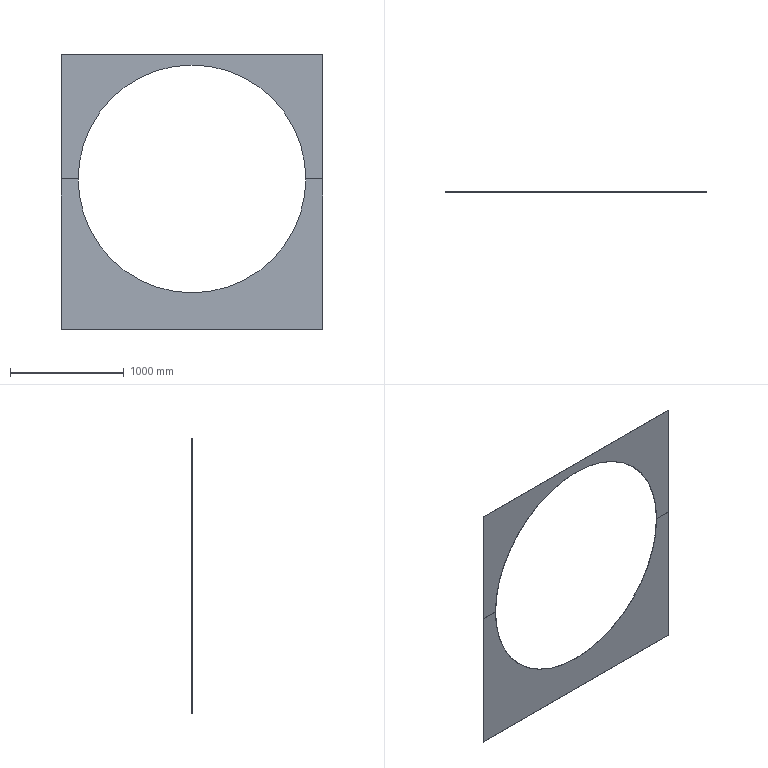Part | STEP file | Bracket checkered plate 8 | 2 solids | 17 faces | box 2300 x 3 x 2420 mm | volume 7273222 mm3 | plane 14 | cylinder 3 | commonest cylinder face diameters 2000 x3
STEP:
#1=CARTESIAN_POINT('',(0.,0.,0.));
#2=DIRECTION('',(0.,0.,1.));
#3=DIRECTION('',(1.,0.,0.));
#4=AXIS2_PLACEMENT_3D('',#1,#2,#3);
#5=CARTESIAN_POINT('',(2150.,3.,-1095.));
#6=VERTEX_POINT('',#5);
#7=CARTESIAN_POINT('',(2150.,0.,-1095.));
#8=VERTEX_POINT('',#7);
#9=CARTESIAN_POINT('',(2150.,-7.,-1095.));
#10=DIRECTION('',(0.,-1.,0.));
#11=VECTOR('',#10,1.);
#12=LINE('',#9,#11);
#13=CARTESIAN_POINT('',(1150.,-7.,-1095.));
#14=DIRECTION('',(0.,1.,0.));
#15=DIRECTION('',(0.,0.,1.));
#16=AXIS2_PLACEMENT_3D('',#13,#14,#15);
#17=CYLINDRICAL_SURFACE('',#16,1000.);
#18=CARTESIAN_POINT('',(1.571,0.));
#19=DIRECTION('',(0.,-1.));
#20=VECTOR('',#19,1.);
#21=LINE('',#18,#20);
#22=(GEOMETRIC_REPRESENTATION_CONTEXT(2)PARAMETRIC_REPRESENTATION_CONTEXT()REPRESENTATION_CONTEXT('',''));
#23=DEFINITIONAL_REPRESENTATION('',(#21),#22);
#24=PCURVE('',#17,#23);
#25=CARTESIAN_POINT('',(0.,-0.01,-1095.));
#26=DIRECTION('',(0.,0.,1.));
#27=DIRECTION('',(1.,0.,0.));
#28=AXIS2_PLACEMENT_3D('',#25,#26,#27);
#29=PLANE('',#28);
#30=CARTESIAN_POINT('',(2150.,-6.99));
#31=DIRECTION('',(0.,-1.));
#32=VECTOR('',#31,1.);
#33=LINE('',#30,#32);
#34=(GEOMETRIC_REPRESENTATION_CONTEXT(2)PARAMETRIC_REPRESENTATION_CONTEXT()REPRESENTATION_CONTEXT('',''));
#35=DEFINITIONAL_REPRESENTATION('',(#33),#34);
#36=PCURVE('',#29,#35);
#37=SURFACE_CURVE('',#12,(#24,#36),.PCURVE_S1.);
#38=EDGE_CURVE('',#6,#8,#37,.T.);
#39=ORIENTED_EDGE('',*,*,#38,.F.);
#40=CARTESIAN_POINT('',(1150.,3.,-95.));
#41=VERTEX_POINT('',#40);
#42=CARTESIAN_POINT('',(1150.,3.,-1095.));
#43=DIRECTION('',(0.,1.,0.));
#44=DIRECTION('',(0.,0.,1.));
#45=AXIS2_PLACEMENT_3D('',#42,#43,#44);
#46=CIRCLE('',#45,1000.);
#47=CARTESIAN_POINT('',(0.,10.));
#48=DIRECTION('',(1.,0.));
#49=VECTOR('',#48,1.);
#50=LINE('',#47,#49);
#51=(GEOMETRIC_REPRESENTATION_CONTEXT(2)PARAMETRIC_REPRESENTATION_CONTEXT()REPRESENTATION_CONTEXT('',''));
#52=DEFINITIONAL_REPRESENTATION('',(#50),#51);
#53=PCURVE('',#17,#52);
#54=CARTESIAN_POINT('',(0.,3.,0.));
#55=DIRECTION('',(0.,-1.,0.));
#56=DIRECTION('',(0.,0.,-1.));
#57=AXIS2_PLACEMENT_3D('',#54,#55,#56);
#58=PLANE('',#57);
#59=CARTESIAN_POINT('',(95.,1150.));
#60=CARTESIAN_POINT('',(95.,2882.051));
#61=CARTESIAN_POINT('',(1595.,2016.025));
#62=CARTESIAN_POINT('',(3095.,1150.));
#63=CARTESIAN_POINT('',(1595.,283.975));
#64=CARTESIAN_POINT('',(95.,-582.051));
#65=CARTESIAN_POINT('',(95.,1150.));
#66=(BOUNDED_CURVE()B_SPLINE_CURVE(2,(#59,#60,#61,#62,#63,#64,#65),.UNSPECIFIED.,.T.,.F.)B_SPLINE_CURVE_WITH_KNOTS((1,2,2,2,2,1),(-2.094,0.,2.094,4.189,6.283,8.378),.UNSPECIFIED.)CURVE()GEOMETRIC_REPRESENTATION_ITEM()RATIONAL_B_SPLINE_CURVE((1.,0.5,1.,0.5,1.,0.5,1.))REPRESENTATION_ITEM(''));
#67=(GEOMETRIC_REPRESENTATION_CONTEXT(2)PARAMETRIC_REPRESENTATION_CONTEXT()REPRESENTATION_CONTEXT('',''));
#68=DEFINITIONAL_REPRESENTATION('',(#66),#67);
#69=PCURVE('',#58,#68);
#70=SURFACE_CURVE('',#46,(#53,#69),.PCURVE_S1.);
#71=EDGE_CURVE('',#41,#6,#70,.T.);
#72=ORIENTED_EDGE('',*,*,#71,.F.);
#73=CARTESIAN_POINT('',(1150.,0.,-95.));
#74=VERTEX_POINT('',#73);
#75=CARTESIAN_POINT('',(1150.,-7.,-95.));
#76=DIRECTION('',(0.,1.,0.));
#77=VECTOR('',#76,1.);
#78=LINE('',#75,#77);
#79=CARTESIAN_POINT('',(0.,0.));
#80=DIRECTION('',(0.,1.));
#81=VECTOR('',#80,1.);
#82=LINE('',#79,#81);
#83=(GEOMETRIC_REPRESENTATION_CONTEXT(2)PARAMETRIC_REPRESENTATION_CONTEXT()REPRESENTATION_CONTEXT('',''));
#84=DEFINITIONAL_REPRESENTATION('',(#82),#83);
#85=PCURVE('',#17,#84);
#86=CARTESIAN_POINT('',(1150.,-7.,-1095.));
#87=DIRECTION('',(0.,1.,0.));
#88=DIRECTION('',(0.,0.,1.));
#89=AXIS2_PLACEMENT_3D('',#86,#87,#88);
#90=CYLINDRICAL_SURFACE('',#89,1000.);
#91=CARTESIAN_POINT('',(6.283,0.));
#92=DIRECTION('',(0.,1.));
#93=VECTOR('',#92,1.);
#94=LINE('',#91,#93);
#95=(GEOMETRIC_REPRESENTATION_CONTEXT(2)PARAMETRIC_REPRESENTATION_CONTEXT()REPRESENTATION_CONTEXT('',''));
#96=DEFINITIONAL_REPRESENTATION('',(#94),#95);
#97=PCURVE('',#90,#96);
#98=SURFACE_CURVE('',#78,(#85,#97),.PCURVE_S1.);
#99=EDGE_CURVE('',#74,#41,#98,.T.);
#100=ORIENTED_EDGE('',*,*,#99,.F.);
#101=CARTESIAN_POINT('',(1150.,0.,-1095.));
#102=DIRECTION('',(0.,-1.,0.));
#103=DIRECTION('',(0.,0.,-1.));
#104=AXIS2_PLACEMENT_3D('',#101,#102,#103);
#105=CIRCLE('',#104,1000.);
#106=CARTESIAN_POINT('',(3.142,7.));
#107=DIRECTION('',(-1.,0.));
#108=VECTOR('',#107,1.);
#109=LINE('',#106,#108);
#110=(GEOMETRIC_REPRESENTATION_CONTEXT(2)PARAMETRIC_REPRESENTATION_CONTEXT()REPRESENTATION_CONTEXT('',''));
#111=DEFINITIONAL_REPRESENTATION('',(#109),#110);
#112=PCURVE('',#17,#111);
#113=CARTESIAN_POINT('',(0.,0.,0.));
#114=DIRECTION('',(0.,-1.,0.));
#115=DIRECTION('',(0.,0.,-1.));
#116=AXIS2_PLACEMENT_3D('',#113,#114,#115);
#117=PLANE('',#116);
#118=CARTESIAN_POINT('',(1095.,1150.));
#119=DIRECTION('',(1.,0.));
#120=AXIS2_PLACEMENT_2D('',#118,#119);
#121=CIRCLE('',#120,1000.);
#122=(GEOMETRIC_REPRESENTATION_CONTEXT(2)PARAMETRIC_REPRESENTATION_CONTEXT()REPRESENTATION_CONTEXT('',''));
#123=DEFINITIONAL_REPRESENTATION('',(#121),#122);
#124=PCURVE('',#117,#123);
#125=SURFACE_CURVE('',#105,(#112,#124),.PCURVE_S1.);
#126=EDGE_CURVE('',#8,#74,#125,.T.);
#127=ORIENTED_EDGE('',*,*,#126,.F.);
#128=EDGE_LOOP('',(#39,#72,#100,#127));
#129=FACE_BOUND('',#128,.F.);
#130=ADVANCED_FACE('',(#129),#17,.F.);
#131=CARTESIAN_POINT('',(2300.,0.,-1095.));
#132=VERTEX_POINT('',#131);
#133=CARTESIAN_POINT('',(0.,0.,-1095.));
#134=DIRECTION('',(-1.,0.,0.));
#135=VECTOR('',#134,1.);
#136=LINE('',#133,#135);
#137=CARTESIAN_POINT('',(0.,0.01));
#138=DIRECTION('',(-1.,0.));
#139=VECTOR('',#138,1.);
#140=LINE('',#137,#139);
#141=(GEOMETRIC_REPRESENTATION_CONTEXT(2)PARAMETRIC_REPRESENTATION_CONTEXT()REPRESENTATION_CONTEXT('',''));
#142=DEFINITIONAL_REPRESENTATION('',(#140),#141);
#143=PCURVE('',#29,#142);
#144=CARTESIAN_POINT('',(1095.,0.));
#145=DIRECTION('',(0.,-1.));
#146=VECTOR('',#145,1.);
#147=LINE('',#144,#146);
#148=(GEOMETRIC_REPRESENTATION_CONTEXT(2)PARAMETRIC_REPRESENTATION_CONTEXT()REPRESENTATION_CONTEXT('',''));
#149=DEFINITIONAL_REPRESENTATION('',(#147),#148);
#150=PCURVE('',#117,#149);
#151=SURFACE_CURVE('',#136,(#143,#150),.PCURVE_S1.);
#152=EDGE_CURVE('',#132,#8,#151,.T.);
#153=ORIENTED_EDGE('',*,*,#152,.T.);
#154=ORIENTED_EDGE('',*,*,#38,.F.);
#155=CARTESIAN_POINT('',(2300.,3.,-1095.));
#156=VERTEX_POINT('',#155);
#157=CARTESIAN_POINT('',(0.,3.,-1095.));
#158=DIRECTION('',(-1.,0.,0.));
#159=VECTOR('',#158,1.);
#160=LINE('',#157,#159);
#161=CARTESIAN_POINT('',(0.,3.01));
#162=DIRECTION('',(-1.,0.));
#163=VECTOR('',#162,1.);
#164=LINE('',#161,#163);
#165=(GEOMETRIC_REPRESENTATION_CONTEXT(2)PARAMETRIC_REPRESENTATION_CONTEXT()REPRESENTATION_CONTEXT('',''));
#166=DEFINITIONAL_REPRESENTATION('',(#164),#165);
#167=PCURVE('',#29,#166);
#168=CARTESIAN_POINT('',(1095.,0.));
#169=DIRECTION('',(0.,-1.));
#170=VECTOR('',#169,1.);
#171=LINE('',#168,#170);
#172=(GEOMETRIC_REPRESENTATION_CONTEXT(2)PARAMETRIC_REPRESENTATION_CONTEXT()REPRESENTATION_CONTEXT('',''));
#173=DEFINITIONAL_REPRESENTATION('',(#171),#172);
#174=PCURVE('',#58,#173);
#175=SURFACE_CURVE('',#160,(#167,#174),.PCURVE_S1.);
#176=EDGE_CURVE('',#156,#6,#175,.T.);
#177=ORIENTED_EDGE('',*,*,#176,.F.);
#178=CARTESIAN_POINT('',(2300.,3.,-1095.));
#179=DIRECTION('',(0.,1.,0.));
#180=VECTOR('',#179,1.);
#181=LINE('',#178,#180);
#182=CARTESIAN_POINT('',(2300.,3.01));
#183=DIRECTION('',(0.,1.));
#184=VECTOR('',#183,1.);
#185=LINE('',#182,#184);
#186=(GEOMETRIC_REPRESENTATION_CONTEXT(2)PARAMETRIC_REPRESENTATION_CONTEXT()REPRESENTATION_CONTEXT('',''));
#187=DEFINITIONAL_REPRESENTATION('',(#185),#186);
#188=PCURVE('',#29,#187);
#189=CARTESIAN_POINT('',(2300.,3.,0.));
#190=DIRECTION('',(-1.,0.,0.));
#191=DIRECTION('',(0.,0.,1.));
#192=AXIS2_PLACEMENT_3D('',#189,#190,#191);
#193=PLANE('',#192);
#194=CARTESIAN_POINT('',(-1095.,0.));
#195=DIRECTION('',(0.,1.));
#196=VECTOR('',#195,1.);
#197=LINE('',#194,#196);
#198=(GEOMETRIC_REPRESENTATION_CONTEXT(2)PARAMETRIC_REPRESENTATION_CONTEXT()REPRESENTATION_CONTEXT('',''));
#199=DEFINITIONAL_REPRESENTATION('',(#197),#198);
#200=PCURVE('',#193,#199);
#201=SURFACE_CURVE('',#181,(#188,#200),.PCURVE_S1.);
#202=EDGE_CURVE('',#132,#156,#201,.T.);
#203=ORIENTED_EDGE('',*,*,#202,.F.);
#204=EDGE_LOOP('',(#153,#154,#177,#203));
#205=FACE_BOUND('',#204,.T.);
#206=ADVANCED_FACE('',(#205),#29,.F.);
#207=CARTESIAN_POINT('',(150.,0.,-1095.));
#208=VERTEX_POINT('',#207);
#209=CARTESIAN_POINT('',(0.,0.,-1095.));
#210=VERTEX_POINT('',#209);
#211=CARTESIAN_POINT('',(0.,0.,-1095.));
#212=DIRECTION('',(-1.,0.,0.));
#213=VECTOR('',#212,1.);
#214=LINE('',#211,#213);
#215=CARTESIAN_POINT('',(0.,-0.01,-1095.));
#216=DIRECTION('',(0.,0.,1.));
#217=DIRECTION('',(1.,0.,0.));
#218=AXIS2_PLACEMENT_3D('',#215,#216,#217);
#219=PLANE('',#218);
#220=CARTESIAN_POINT('',(0.,0.01));
#221=DIRECTION('',(-1.,0.));
#222=VECTOR('',#221,1.);
#223=LINE('',#220,#222);
#224=(GEOMETRIC_REPRESENTATION_CONTEXT(2)PARAMETRIC_REPRESENTATION_CONTEXT()REPRESENTATION_CONTEXT('',''));
#225=DEFINITIONAL_REPRESENTATION('',(#223),#224);
#226=PCURVE('',#219,#225);
#227=CARTESIAN_POINT('',(1095.,0.));
#228=DIRECTION('',(0.,-1.));
#229=VECTOR('',#228,1.);
#230=LINE('',#227,#229);
#231=(GEOMETRIC_REPRESENTATION_CONTEXT(2)PARAMETRIC_REPRESENTATION_CONTEXT()REPRESENTATION_CONTEXT('',''));
#232=DEFINITIONAL_REPRESENTATION('',(#230),#231);
#233=PCURVE('',#117,#232);
#234=SURFACE_CURVE('',#214,(#226,#233),.PCURVE_S1.);
#235=EDGE_CURVE('',#208,#210,#234,.T.);
#236=ORIENTED_EDGE('',*,*,#235,.T.);
#237=CARTESIAN_POINT('',(0.,3.,-1095.));
#238=VERTEX_POINT('',#237);
#239=CARTESIAN_POINT('',(0.,3.,-1095.));
#240=DIRECTION('',(0.,-1.,0.));
#241=VECTOR('',#240,1.);
#242=LINE('',#239,#241);
#243=CARTESIAN_POINT('',(0.,3.01));
#244=DIRECTION('',(0.,-1.));
#245=VECTOR('',#244,1.);
#246=LINE('',#243,#245);
#247=(GEOMETRIC_REPRESENTATION_CONTEXT(2)PARAMETRIC_REPRESENTATION_CONTEXT()REPRESENTATION_CONTEXT('',''));
#248=DEFINITIONAL_REPRESENTATION('',(#246),#247);
#249=PCURVE('',#219,#248);
#250=CARTESIAN_POINT('',(0.,3.,0.));
#251=DIRECTION('',(1.,0.,0.));
#252=DIRECTION('',(0.,0.,-1.));
#253=AXIS2_PLACEMENT_3D('',#250,#251,#252);
#254=PLANE('',#253);
#255=CARTESIAN_POINT('',(1095.,0.));
#256=DIRECTION('',(0.,-1.));
#257=VECTOR('',#256,1.);
#258=LINE('',#255,#257);
#259=(GEOMETRIC_REPRESENTATION_CONTEXT(2)PARAMETRIC_REPRESENTATION_CONTEXT()REPRESENTATION_CONTEXT('',''));
#260=DEFINITIONAL_REPRESENTATION('',(#258),#259);
#261=PCURVE('',#254,#260);
#262=SURFACE_CURVE('',#242,(#249,#261),.PCURVE_S1.);
#263=EDGE_CURVE('',#238,#210,#262,.T.);
#264=ORIENTED_EDGE('',*,*,#263,.F.);
#265=CARTESIAN_POINT('',(150.,3.,-1095.));
#266=VERTEX_POINT('',#265);
#267=CARTESIAN_POINT('',(0.,3.,-1095.));
#268=DIRECTION('',(-1.,0.,0.));
#269=VECTOR('',#268,1.);
#270=LINE('',#267,#269);
#271=CARTESIAN_POINT('',(0.,3.01));
#272=DIRECTION('',(-1.,0.));
#273=VECTOR('',#272,1.);
#274=LINE('',#271,#273);
#275=(GEOMETRIC_REPRESENTATION_CONTEXT(2)PARAMETRIC_REPRESENTATION_CONTEXT()REPRESENTATION_CONTEXT('',''));
#276=DEFINITIONAL_REPRESENTATION('',(#274),#275);
#277=PCURVE('',#219,#276);
#278=CARTESIAN_POINT('',(1095.,0.));
#279=DIRECTION('',(0.,-1.));
#280=VECTOR('',#279,1.);
#281=LINE('',#278,#280);
#282=(GEOMETRIC_REPRESENTATION_CONTEXT(2)PARAMETRIC_REPRESENTATION_CONTEXT()REPRESENTATION_CONTEXT('',''));
#283=DEFINITIONAL_REPRESENTATION('',(#281),#282);
#284=PCURVE('',#58,#283);
#285=SURFACE_CURVE('',#270,(#277,#284),.PCURVE_S1.);
#286=EDGE_CURVE('',#266,#238,#285,.T.);
#287=ORIENTED_EDGE('',*,*,#286,.F.);
#288=CARTESIAN_POINT('',(150.,-7.,-1095.));
#289=DIRECTION('',(0.,1.,0.));
#290=VECTOR('',#289,1.);
#291=LINE('',#288,#290);
#292=CARTESIAN_POINT('',(150.,-6.99));
#293=DIRECTION('',(0.,1.));
#294=VECTOR('',#293,1.);
#295=LINE('',#292,#294);
#296=(GEOMETRIC_REPRESENTATION_CONTEXT(2)PARAMETRIC_REPRESENTATION_CONTEXT()REPRESENTATION_CONTEXT('',''));
#297=DEFINITIONAL_REPRESENTATION('',(#295),#296);
#298=PCURVE('',#219,#297);
#299=CARTESIAN_POINT('',(4.712,0.));
#300=DIRECTION('',(0.,1.));
#301=VECTOR('',#300,1.);
#302=LINE('',#299,#301);
#303=(GEOMETRIC_REPRESENTATION_CONTEXT(2)PARAMETRIC_REPRESENTATION_CONTEXT()REPRESENTATION_CONTEXT('',''));
#304=DEFINITIONAL_REPRESENTATION('',(#302),#303);
#305=PCURVE('',#90,#304);
#306=SURFACE_CURVE('',#291,(#298,#305),.PCURVE_S1.);
#307=EDGE_CURVE('',#208,#266,#306,.T.);
#308=ORIENTED_EDGE('',*,*,#307,.F.);
#309=EDGE_LOOP('',(#236,#264,#287,#308));
#310=FACE_BOUND('',#309,.T.);
#311=ADVANCED_FACE('',(#310),#219,.F.);
#312=CARTESIAN_POINT('',(1150.,3.,-1095.));
#313=DIRECTION('',(0.,1.,0.));
#314=DIRECTION('',(0.,0.,1.));
#315=AXIS2_PLACEMENT_3D('',#312,#313,#314);
#316=CIRCLE('',#315,1000.);
#317=CARTESIAN_POINT('',(0.,10.));
#318=DIRECTION('',(1.,0.));
#319=VECTOR('',#318,1.);
#320=LINE('',#317,#319);
#321=(GEOMETRIC_REPRESENTATION_CONTEXT(2)PARAMETRIC_REPRESENTATION_CONTEXT()REPRESENTATION_CONTEXT('',''));
#322=DEFINITIONAL_REPRESENTATION('',(#320),#321);
#323=PCURVE('',#90,#322);
#324=CARTESIAN_POINT('',(95.,1150.));
#325=CARTESIAN_POINT('',(95.,2882.051));
#326=CARTESIAN_POINT('',(1595.,2016.025));
#327=CARTESIAN_POINT('',(3095.,1150.));
#328=CARTESIAN_POINT('',(1595.,283.975));
#329=CARTESIAN_POINT('',(95.,-582.051));
#330=CARTESIAN_POINT('',(95.,1150.));
#331=(BOUNDED_CURVE()B_SPLINE_CURVE(2,(#324,#325,#326,#327,#328,#329,#330),.UNSPECIFIED.,.T.,.F.)B_SPLINE_CURVE_WITH_KNOTS((1,2,2,2,2,1),(-2.094,0.,2.094,4.189,6.283,8.378),.UNSPECIFIED.)CURVE()GEOMETRIC_REPRESENTATION_ITEM()RATIONAL_B_SPLINE_CURVE((1.,0.5,1.,0.5,1.,0.5,1.))REPRESENTATION_ITEM(''));
#332=(GEOMETRIC_REPRESENTATION_CONTEXT(2)PARAMETRIC_REPRESENTATION_CONTEXT()REPRESENTATION_CONTEXT('',''));
#333=DEFINITIONAL_REPRESENTATION('',(#331),#332);
#334=PCURVE('',#58,#333);
#335=SURFACE_CURVE('',#316,(#323,#334),.PCURVE_S1.);
#336=EDGE_CURVE('',#266,#41,#335,.T.);
#337=ORIENTED_EDGE('',*,*,#336,.F.);
#338=ORIENTED_EDGE('',*,*,#307,.F.);
#339=CARTESIAN_POINT('',(1150.,0.,-1095.));
#340=DIRECTION('',(0.,-1.,0.));
#341=DIRECTION('',(0.,0.,-1.));
#342=AXIS2_PLACEMENT_3D('',#339,#340,#341);
#343=CIRCLE('',#342,1000.);
#344=CARTESIAN_POINT('',(9.425,7.));
#345=DIRECTION('',(-1.,0.));
#346=VECTOR('',#345,1.);
#347=LINE('',#344,#346);
#348=(GEOMETRIC_REPRESENTATION_CONTEXT(2)PARAMETRIC_REPRESENTATION_CONTEXT()REPRESENTATION_CONTEXT('',''));
#349=DEFINITIONAL_REPRESENTATION('',(#347),#348);
#350=PCURVE('',#90,#349);
#351=CARTESIAN_POINT('',(1095.,1150.));
#352=DIRECTION('',(1.,0.));
#353=AXIS2_PLACEMENT_2D('',#351,#352);
#354=CIRCLE('',#353,1000.);
#355=(GEOMETRIC_REPRESENTATION_CONTEXT(2)PARAMETRIC_REPRESENTATION_CONTEXT()REPRESENTATION_CONTEXT('',''));
#356=DEFINITIONAL_REPRESENTATION('',(#354),#355);
#357=PCURVE('',#117,#356);
#358=SURFACE_CURVE('',#343,(#350,#357),.PCURVE_S1.);
#359=EDGE_CURVE('',#74,#208,#358,.T.);
#360=ORIENTED_EDGE('',*,*,#359,.F.);
#361=ORIENTED_EDGE('',*,*,#99,.T.);
#362=EDGE_LOOP('',(#337,#338,#360,#361));
#363=FACE_BOUND('',#362,.F.);
#364=ADVANCED_FACE('',(#363),#90,.F.);
#365=CARTESIAN_POINT('',(2300.,3.,0.));
#366=VERTEX_POINT('',#365);
#367=CARTESIAN_POINT('',(2300.,3.,0.));
#368=DIRECTION('',(0.,0.,-1.));
#369=VECTOR('',#368,1.);
#370=LINE('',#367,#369);
#371=CARTESIAN_POINT('',(0.,2300.));
#372=DIRECTION('',(1.,0.));
#373=VECTOR('',#372,1.);
#374=LINE('',#371,#373);
#375=(GEOMETRIC_REPRESENTATION_CONTEXT(2)PARAMETRIC_REPRESENTATION_CONTEXT()REPRESENTATION_CONTEXT('',''));
#376=DEFINITIONAL_REPRESENTATION('',(#374),#375);
#377=PCURVE('',#58,#376);
#378=CARTESIAN_POINT('',(0.,0.));
#379=DIRECTION('',(-1.,0.));
#380=VECTOR('',#379,1.);
#381=LINE('',#378,#380);
#382=(GEOMETRIC_REPRESENTATION_CONTEXT(2)PARAMETRIC_REPRESENTATION_CONTEXT()REPRESENTATION_CONTEXT('',''));
#383=DEFINITIONAL_REPRESENTATION('',(#381),#382);
#384=PCURVE('',#193,#383);
#385=SURFACE_CURVE('',#370,(#377,#384),.PCURVE_S1.);
#386=EDGE_CURVE('',#366,#156,#385,.T.);
#387=ORIENTED_EDGE('',*,*,#386,.T.);
#388=ORIENTED_EDGE('',*,*,#176,.T.);
#389=ORIENTED_EDGE('',*,*,#71,.F.);
#390=ORIENTED_EDGE('',*,*,#336,.F.);
#391=ORIENTED_EDGE('',*,*,#286,.T.);
#392=CARTESIAN_POINT('',(0.,3.,0.));
#393=VERTEX_POINT('',#392);
#394=CARTESIAN_POINT('',(0.,3.,0.));
#395=DIRECTION('',(0.,0.,1.));
#396=VECTOR('',#395,1.);
#397=LINE('',#394,#396);
#398=CARTESIAN_POINT('',(0.,0.));
#399=DIRECTION('',(-1.,0.));
#400=VECTOR('',#399,1.);
#401=LINE('',#398,#400);
#402=(GEOMETRIC_REPRESENTATION_CONTEXT(2)PARAMETRIC_REPRESENTATION_CONTEXT()REPRESENTATION_CONTEXT('',''));
#403=DEFINITIONAL_REPRESENTATION('',(#401),#402);
#404=PCURVE('',#58,#403);
#405=CARTESIAN_POINT('',(0.,0.));
#406=DIRECTION('',(-1.,0.));
#407=VECTOR('',#406,1.);
#408=LINE('',#405,#407);
#409=(GEOMETRIC_REPRESENTATION_CONTEXT(2)PARAMETRIC_REPRESENTATION_CONTEXT()REPRESENTATION_CONTEXT('',''));
#410=DEFINITIONAL_REPRESENTATION('',(#408),#409);
#411=PCURVE('',#254,#410);
#412=SURFACE_CURVE('',#397,(#404,#411),.PCURVE_S1.);
#413=EDGE_CURVE('',#238,#393,#412,.T.);
#414=ORIENTED_EDGE('',*,*,#413,.T.);
#415=CARTESIAN_POINT('',(0.,3.,0.));
#416=DIRECTION('',(1.,0.,0.));
#417=VECTOR('',#416,1.);
#418=LINE('',#415,#417);
#419=CARTESIAN_POINT('',(0.,0.));
#420=DIRECTION('',(0.,1.));
#421=VECTOR('',#420,1.);
#422=LINE('',#419,#421);
#423=(GEOMETRIC_REPRESENTATION_CONTEXT(2)PARAMETRIC_REPRESENTATION_CONTEXT()REPRESENTATION_CONTEXT('',''));
#424=DEFINITIONAL_REPRESENTATION('',(#422),#423);
#425=PCURVE('',#58,#424);
#426=CARTESIAN_POINT('',(0.,3.,0.));
#427=DIRECTION('',(0.,0.,-1.));
#428=DIRECTION('',(-1.,0.,0.));
#429=AXIS2_PLACEMENT_3D('',#426,#427,#428);
#430=PLANE('',#429);
#431=CARTESIAN_POINT('',(0.,0.));
#432=DIRECTION('',(-1.,0.));
#433=VECTOR('',#432,1.);
#434=LINE('',#431,#433);
#435=(GEOMETRIC_REPRESENTATION_CONTEXT(2)PARAMETRIC_REPRESENTATION_CONTEXT()REPRESENTATION_CONTEXT('',''));
#436=DEFINITIONAL_REPRESENTATION('',(#434),#435);
#437=PCURVE('',#430,#436);
#438=SURFACE_CURVE('',#418,(#425,#437),.PCURVE_S1.);
#439=EDGE_CURVE('',#393,#366,#438,.T.);
#440=ORIENTED_EDGE('',*,*,#439,.T.);
#441=EDGE_LOOP('',(#387,#388,#389,#390,#391,#414,#440));
#442=FACE_BOUND('',#441,.T.);
#443=ADVANCED_FACE('',(#442),#58,.F.);
#444=ORIENTED_EDGE('',*,*,#152,.F.);
#445=CARTESIAN_POINT('',(2300.,0.,0.));
#446=VERTEX_POINT('',#445);
#447=CARTESIAN_POINT('',(2300.,0.,0.));
#448=DIRECTION('',(0.,0.,-1.));
#449=VECTOR('',#448,1.);
#450=LINE('',#447,#449);
#451=CARTESIAN_POINT('',(0.,2300.));
#452=DIRECTION('',(1.,0.));
#453=VECTOR('',#452,1.);
#454=LINE('',#451,#453);
#455=(GEOMETRIC_REPRESENTATION_CONTEXT(2)PARAMETRIC_REPRESENTATION_CONTEXT()REPRESENTATION_CONTEXT('',''));
#456=DEFINITIONAL_REPRESENTATION('',(#454),#455);
#457=PCURVE('',#117,#456);
#458=CARTESIAN_POINT('',(0.,-3.));
#459=DIRECTION('',(-1.,0.));
#460=VECTOR('',#459,1.);
#461=LINE('',#458,#460);
#462=(GEOMETRIC_REPRESENTATION_CONTEXT(2)PARAMETRIC_REPRESENTATION_CONTEXT()REPRESENTATION_CONTEXT('',''));
#463=DEFINITIONAL_REPRESENTATION('',(#461),#462);
#464=PCURVE('',#193,#463);
#465=SURFACE_CURVE('',#450,(#457,#464),.PCURVE_S1.);
#466=EDGE_CURVE('',#446,#132,#465,.T.);
#467=ORIENTED_EDGE('',*,*,#466,.F.);
#468=CARTESIAN_POINT('',(0.,0.,0.));
#469=VERTEX_POINT('',#468);
#470=CARTESIAN_POINT('',(0.,0.,0.));
#471=DIRECTION('',(1.,0.,0.));
#472=VECTOR('',#471,1.);
#473=LINE('',#470,#472);
#474=CARTESIAN_POINT('',(0.,0.));
#475=DIRECTION('',(0.,1.));
#476=VECTOR('',#475,1.);
#477=LINE('',#474,#476);
#478=(GEOMETRIC_REPRESENTATION_CONTEXT(2)PARAMETRIC_REPRESENTATION_CONTEXT()REPRESENTATION_CONTEXT('',''));
#479=DEFINITIONAL_REPRESENTATION('',(#477),#478);
#480=PCURVE('',#117,#479);
#481=CARTESIAN_POINT('',(0.,-3.));
#482=DIRECTION('',(-1.,0.));
#483=VECTOR('',#482,1.);
#484=LINE('',#481,#483);
#485=(GEOMETRIC_REPRESENTATION_CONTEXT(2)PARAMETRIC_REPRESENTATION_CONTEXT()REPRESENTATION_CONTEXT('',''));
#486=DEFINITIONAL_REPRESENTATION('',(#484),#485);
#487=PCURVE('',#430,#486);
#488=SURFACE_CURVE('',#473,(#480,#487),.PCURVE_S1.);
#489=EDGE_CURVE('',#469,#446,#488,.T.);
#490=ORIENTED_EDGE('',*,*,#489,.F.);
#491=CARTESIAN_POINT('',(0.,0.,0.));
#492=DIRECTION('',(0.,0.,1.));
#493=VECTOR('',#492,1.);
#494=LINE('',#491,#493);
#495=CARTESIAN_POINT('',(0.,0.));
#496=DIRECTION('',(-1.,0.));
#497=VECTOR('',#496,1.);
#498=LINE('',#495,#497);
#499=(GEOMETRIC_REPRESENTATION_CONTEXT(2)PARAMETRIC_REPRESENTATION_CONTEXT()REPRESENTATION_CONTEXT('',''));
#500=DEFINITIONAL_REPRESENTATION('',(#498),#499);
#501=PCURVE('',#117,#500);
#502=CARTESIAN_POINT('',(0.,-3.));
#503=DIRECTION('',(-1.,0.));
#504=VECTOR('',#503,1.);
#505=LINE('',#502,#504);
#506=(GEOMETRIC_REPRESENTATION_CONTEXT(2)PARAMETRIC_REPRESENTATION_CONTEXT()REPRESENTATION_CONTEXT('',''));
#507=DEFINITIONAL_REPRESENTATION('',(#505),#506);
#508=PCURVE('',#254,#507);
#509=SURFACE_CURVE('',#494,(#501,#508),.PCURVE_S1.);
#510=EDGE_CURVE('',#210,#469,#509,.T.);
#511=ORIENTED_EDGE('',*,*,#510,.F.);
#512=ORIENTED_EDGE('',*,*,#235,.F.);
#513=ORIENTED_EDGE('',*,*,#359,.F.);
#514=ORIENTED_EDGE('',*,*,#126,.F.);
#515=EDGE_LOOP('',(#444,#467,#490,#511,#512,#513,#514));
#516=FACE_BOUND('',#515,.T.);
#517=ADVANCED_FACE('',(#516),#117,.T.);
#518=ORIENTED_EDGE('',*,*,#466,.T.);
#519=ORIENTED_EDGE('',*,*,#202,.T.);
#520=ORIENTED_EDGE('',*,*,#386,.F.);
#521=CARTESIAN_POINT('',(2300.,3.,0.));
#522=DIRECTION('',(0.,-1.,0.));
#523=VECTOR('',#522,1.);
#524=LINE('',#521,#523);
#525=CARTESIAN_POINT('',(0.,0.));
#526=DIRECTION('',(0.,-1.));
#527=VECTOR('',#526,1.);
#528=LINE('',#525,#527);
#529=(GEOMETRIC_REPRESENTATION_CONTEXT(2)PARAMETRIC_REPRESENTATION_CONTEXT()REPRESENTATION_CONTEXT('',''));
#530=DEFINITIONAL_REPRESENTATION('',(#528),#529);
#531=PCURVE('',#193,#530);
#532=CARTESIAN_POINT('',(-2300.,0.));
#533=DIRECTION('',(0.,-1.));
#534=VECTOR('',#533,1.);
#535=LINE('',#532,#534);
#536=(GEOMETRIC_REPRESENTATION_CONTEXT(2)PARAMETRIC_REPRESENTATION_CONTEXT()REPRESENTATION_CONTEXT('',''));
#537=DEFINITIONAL_REPRESENTATION('',(#535),#536);
#538=PCURVE('',#430,#537);
#539=SURFACE_CURVE('',#524,(#531,#538),.PCURVE_S1.);
#540=EDGE_CURVE('',#366,#446,#539,.T.);
#541=ORIENTED_EDGE('',*,*,#540,.T.);
#542=EDGE_LOOP('',(#518,#519,#520,#541));
#543=FACE_BOUND('',#542,.T.);
#544=ADVANCED_FACE('',(#543),#193,.F.);
#545=ORIENTED_EDGE('',*,*,#489,.T.);
#546=ORIENTED_EDGE('',*,*,#540,.F.);
#547=ORIENTED_EDGE('',*,*,#439,.F.);
#548=CARTESIAN_POINT('',(0.,3.,0.));
#549=DIRECTION('',(0.,-1.,0.));
#550=VECTOR('',#549,1.);
#551=LINE('',#548,#550);
#552=CARTESIAN_POINT('',(0.,0.));
#553=DIRECTION('',(0.,-1.));
#554=VECTOR('',#553,1.);
#555=LINE('',#552,#554);
#556=(GEOMETRIC_REPRESENTATION_CONTEXT(2)PARAMETRIC_REPRESENTATION_CONTEXT()REPRESENTATION_CONTEXT('',''));
#557=DEFINITIONAL_REPRESENTATION('',(#555),#556);
#558=PCURVE('',#430,#557);
#559=CARTESIAN_POINT('',(0.,0.));
#560=DIRECTION('',(0.,-1.));
#561=VECTOR('',#560,1.);
#562=LINE('',#559,#561);
#563=(GEOMETRIC_REPRESENTATION_CONTEXT(2)PARAMETRIC_REPRESENTATION_CONTEXT()REPRESENTATION_CONTEXT('',''));
#564=DEFINITIONAL_REPRESENTATION('',(#562),#563);
#565=PCURVE('',#254,#564);
#566=SURFACE_CURVE('',#551,(#558,#565),.PCURVE_S1.);
#567=EDGE_CURVE('',#393,#469,#566,.T.);
#568=ORIENTED_EDGE('',*,*,#567,.T.);
#569=EDGE_LOOP('',(#545,#546,#547,#568));
#570=FACE_BOUND('',#569,.T.);
#571=ADVANCED_FACE('',(#570),#430,.F.);
#572=ORIENTED_EDGE('',*,*,#413,.F.);
#573=ORIENTED_EDGE('',*,*,#263,.T.);
#574=ORIENTED_EDGE('',*,*,#510,.T.);
#575=ORIENTED_EDGE('',*,*,#567,.F.);
#576=EDGE_LOOP('',(#572,#573,#574,#575));
#577=FACE_BOUND('',#576,.T.);
#578=ADVANCED_FACE('',(#577),#254,.F.);
#579=CLOSED_SHELL('',(#130,#206,#311,#364,#443,#517,#544,#571,#578));
#580=MANIFOLD_SOLID_BREP('',#579);
#581=CARTESIAN_POINT('',(0.,3.,-1095.));
#582=VERTEX_POINT('',#581);
#583=CARTESIAN_POINT('',(0.,0.,-1095.));
#584=VERTEX_POINT('',#583);
#585=CARTESIAN_POINT('',(0.,3.,-1095.));
#586=DIRECTION('',(0.,-1.,0.));
#587=VECTOR('',#586,1.);
#588=LINE('',#585,#587);
#589=CARTESIAN_POINT('',(0.,3.,0.));
#590=DIRECTION('',(1.,0.,0.));
#591=DIRECTION('',(0.,0.,-1.));
#592=AXIS2_PLACEMENT_3D('',#589,#590,#591);
#593=PLANE('',#592);
#594=CARTESIAN_POINT('',(1095.,0.));
#595=DIRECTION('',(0.,-1.));
#596=VECTOR('',#595,1.);
#597=LINE('',#594,#596);
#598=(GEOMETRIC_REPRESENTATION_CONTEXT(2)PARAMETRIC_REPRESENTATION_CONTEXT()REPRESENTATION_CONTEXT('',''));
#599=DEFINITIONAL_REPRESENTATION('',(#597),#598);
#600=PCURVE('',#593,#599);
#601=CARTESIAN_POINT('',(0.,-0.01,-1095.));
#602=DIRECTION('',(0.,0.,1.));
#603=DIRECTION('',(1.,0.,0.));
#604=AXIS2_PLACEMENT_3D('',#601,#602,#603);
#605=PLANE('',#604);
#606=CARTESIAN_POINT('',(0.,3.01));
#607=DIRECTION('',(0.,-1.));
#608=VECTOR('',#607,1.);
#609=LINE('',#606,#608);
#610=(GEOMETRIC_REPRESENTATION_CONTEXT(2)PARAMETRIC_REPRESENTATION_CONTEXT()REPRESENTATION_CONTEXT('',''));
#611=DEFINITIONAL_REPRESENTATION('',(#609),#610);
#612=PCURVE('',#605,#611);
#613=SURFACE_CURVE('',#588,(#600,#612),.PCURVE_S1.);
#614=EDGE_CURVE('',#582,#584,#613,.T.);
#615=ORIENTED_EDGE('',*,*,#614,.F.);
#616=CARTESIAN_POINT('',(0.,3.,-2420.));
#617=VERTEX_POINT('',#616);
#618=CARTESIAN_POINT('',(0.,3.,0.));
#619=DIRECTION('',(0.,0.,1.));
#620=VECTOR('',#619,1.);
#621=LINE('',#618,#620);
#622=CARTESIAN_POINT('',(0.,0.));
#623=DIRECTION('',(-1.,0.));
#624=VECTOR('',#623,1.);
#625=LINE('',#622,#624);
#626=(GEOMETRIC_REPRESENTATION_CONTEXT(2)PARAMETRIC_REPRESENTATION_CONTEXT()REPRESENTATION_CONTEXT('',''));
#627=DEFINITIONAL_REPRESENTATION('',(#625),#626);
#628=PCURVE('',#593,#627);
#629=CARTESIAN_POINT('',(0.,3.,0.));
#630=DIRECTION('',(0.,-1.,0.));
#631=DIRECTION('',(0.,0.,-1.));
#632=AXIS2_PLACEMENT_3D('',#629,#630,#631);
#633=PLANE('',#632);
#634=CARTESIAN_POINT('',(0.,0.));
#635=DIRECTION('',(-1.,0.));
#636=VECTOR('',#635,1.);
#637=LINE('',#634,#636);
#638=(GEOMETRIC_REPRESENTATION_CONTEXT(2)PARAMETRIC_REPRESENTATION_CONTEXT()REPRESENTATION_CONTEXT('',''));
#639=DEFINITIONAL_REPRESENTATION('',(#637),#638);
#640=PCURVE('',#633,#639);
#641=SURFACE_CURVE('',#621,(#628,#640),.PCURVE_S1.);
#642=EDGE_CURVE('',#617,#582,#641,.T.);
#643=ORIENTED_EDGE('',*,*,#642,.F.);
#644=CARTESIAN_POINT('',(0.,0.,-2420.));
#645=VERTEX_POINT('',#644);
#646=CARTESIAN_POINT('',(0.,3.,-2420.));
#647=DIRECTION('',(0.,-1.,0.));
#648=VECTOR('',#647,1.);
#649=LINE('',#646,#648);
#650=CARTESIAN_POINT('',(2420.,0.));
#651=DIRECTION('',(0.,-1.));
#652=VECTOR('',#651,1.);
#653=LINE('',#650,#652);
#654=(GEOMETRIC_REPRESENTATION_CONTEXT(2)PARAMETRIC_REPRESENTATION_CONTEXT()REPRESENTATION_CONTEXT('',''));
#655=DEFINITIONAL_REPRESENTATION('',(#653),#654);
#656=PCURVE('',#593,#655);
#657=CARTESIAN_POINT('',(0.,3.,-2420.));
#658=DIRECTION('',(0.,0.,1.));
#659=DIRECTION('',(1.,0.,0.));
#660=AXIS2_PLACEMENT_3D('',#657,#658,#659);
#661=PLANE('',#660);
#662=CARTESIAN_POINT('',(0.,0.));
#663=DIRECTION('',(0.,-1.));
#664=VECTOR('',#663,1.);
#665=LINE('',#662,#664);
#666=(GEOMETRIC_REPRESENTATION_CONTEXT(2)PARAMETRIC_REPRESENTATION_CONTEXT()REPRESENTATION_CONTEXT('',''));
#667=DEFINITIONAL_REPRESENTATION('',(#665),#666);
#668=PCURVE('',#661,#667);
#669=SURFACE_CURVE('',#649,(#656,#668),.PCURVE_S1.);
#670=EDGE_CURVE('',#617,#645,#669,.T.);
#671=ORIENTED_EDGE('',*,*,#670,.T.);
#672=CARTESIAN_POINT('',(0.,0.,0.));
#673=DIRECTION('',(0.,0.,1.));
#674=VECTOR('',#673,1.);
#675=LINE('',#672,#674);
#676=CARTESIAN_POINT('',(0.,-3.));
#677=DIRECTION('',(-1.,0.));
#678=VECTOR('',#677,1.);
#679=LINE('',#676,#678);
#680=(GEOMETRIC_REPRESENTATION_CONTEXT(2)PARAMETRIC_REPRESENTATION_CONTEXT()REPRESENTATION_CONTEXT('',''));
#681=DEFINITIONAL_REPRESENTATION('',(#679),#680);
#682=PCURVE('',#593,#681);
#683=CARTESIAN_POINT('',(0.,0.,0.));
#684=DIRECTION('',(0.,-1.,0.));
#685=DIRECTION('',(0.,0.,-1.));
#686=AXIS2_PLACEMENT_3D('',#683,#684,#685);
#687=PLANE('',#686);
#688=CARTESIAN_POINT('',(0.,0.));
#689=DIRECTION('',(-1.,0.));
#690=VECTOR('',#689,1.);
#691=LINE('',#688,#690);
#692=(GEOMETRIC_REPRESENTATION_CONTEXT(2)PARAMETRIC_REPRESENTATION_CONTEXT()REPRESENTATION_CONTEXT('',''));
#693=DEFINITIONAL_REPRESENTATION('',(#691),#692);
#694=PCURVE('',#687,#693);
#695=SURFACE_CURVE('',#675,(#682,#694),.PCURVE_S1.);
#696=EDGE_CURVE('',#645,#584,#695,.T.);
#697=ORIENTED_EDGE('',*,*,#696,.T.);
#698=EDGE_LOOP('',(#615,#643,#671,#697));
#699=FACE_BOUND('',#698,.T.);
#700=ADVANCED_FACE('',(#699),#593,.F.);
#701=CARTESIAN_POINT('',(2300.,0.,-1095.));
#702=VERTEX_POINT('',#701);
#703=CARTESIAN_POINT('',(2300.,3.,-1095.));
#704=VERTEX_POINT('',#703);
#705=CARTESIAN_POINT('',(2300.,3.,-1095.));
#706=DIRECTION('',(0.,1.,0.));
#707=VECTOR('',#706,1.);
#708=LINE('',#705,#707);
#709=CARTESIAN_POINT('',(2300.,3.,0.));
#710=DIRECTION('',(-1.,0.,0.));
#711=DIRECTION('',(0.,0.,1.));
#712=AXIS2_PLACEMENT_3D('',#709,#710,#711);
#713=PLANE('',#712);
#714=CARTESIAN_POINT('',(-1095.,0.));
#715=DIRECTION('',(0.,1.));
#716=VECTOR('',#715,1.);
#717=LINE('',#714,#716);
#718=(GEOMETRIC_REPRESENTATION_CONTEXT(2)PARAMETRIC_REPRESENTATION_CONTEXT()REPRESENTATION_CONTEXT('',''));
#719=DEFINITIONAL_REPRESENTATION('',(#717),#718);
#720=PCURVE('',#713,#719);
#721=CARTESIAN_POINT('',(0.,-0.01,-1095.));
#722=DIRECTION('',(0.,0.,1.));
#723=DIRECTION('',(1.,0.,0.));
#724=AXIS2_PLACEMENT_3D('',#721,#722,#723);
#725=PLANE('',#724);
#726=CARTESIAN_POINT('',(2300.,3.01));
#727=DIRECTION('',(0.,1.));
#728=VECTOR('',#727,1.);
#729=LINE('',#726,#728);
#730=(GEOMETRIC_REPRESENTATION_CONTEXT(2)PARAMETRIC_REPRESENTATION_CONTEXT()REPRESENTATION_CONTEXT('',''));
#731=DEFINITIONAL_REPRESENTATION('',(#729),#730);
#732=PCURVE('',#725,#731);
#733=SURFACE_CURVE('',#708,(#720,#732),.PCURVE_S1.);
#734=EDGE_CURVE('',#702,#704,#733,.T.);
#735=ORIENTED_EDGE('',*,*,#734,.F.);
#736=CARTESIAN_POINT('',(2300.,0.,-2420.));
#737=VERTEX_POINT('',#736);
#738=CARTESIAN_POINT('',(2300.,0.,0.));
#739=DIRECTION('',(0.,0.,-1.));
#740=VECTOR('',#739,1.);
#741=LINE('',#738,#740);
#742=CARTESIAN_POINT('',(0.,-3.));
#743=DIRECTION('',(-1.,0.));
#744=VECTOR('',#743,1.);
#745=LINE('',#742,#744);
#746=(GEOMETRIC_REPRESENTATION_CONTEXT(2)PARAMETRIC_REPRESENTATION_CONTEXT()REPRESENTATION_CONTEXT('',''));
#747=DEFINITIONAL_REPRESENTATION('',(#745),#746);
#748=PCURVE('',#713,#747);
#749=CARTESIAN_POINT('',(0.,2300.));
#750=DIRECTION('',(1.,0.));
#751=VECTOR('',#750,1.);
#752=LINE('',#749,#751);
#753=(GEOMETRIC_REPRESENTATION_CONTEXT(2)PARAMETRIC_REPRESENTATION_CONTEXT()REPRESENTATION_CONTEXT('',''));
#754=DEFINITIONAL_REPRESENTATION('',(#752),#753);
#755=PCURVE('',#687,#754);
#756=SURFACE_CURVE('',#741,(#748,#755),.PCURVE_S1.);
#757=EDGE_CURVE('',#702,#737,#756,.T.);
#758=ORIENTED_EDGE('',*,*,#757,.T.);
#759=CARTESIAN_POINT('',(2300.,3.,-2420.));
#760=VERTEX_POINT('',#759);
#761=CARTESIAN_POINT('',(2300.,3.,-2420.));
#762=DIRECTION('',(0.,-1.,0.));
#763=VECTOR('',#762,1.);
#764=LINE('',#761,#763);
#765=CARTESIAN_POINT('',(-2420.,0.));
#766=DIRECTION('',(0.,-1.));
#767=VECTOR('',#766,1.);
#768=LINE('',#765,#767);
#769=(GEOMETRIC_REPRESENTATION_CONTEXT(2)PARAMETRIC_REPRESENTATION_CONTEXT()REPRESENTATION_CONTEXT('',''));
#770=DEFINITIONAL_REPRESENTATION('',(#768),#769);
#771=PCURVE('',#713,#770);
#772=CARTESIAN_POINT('',(2300.,0.));
#773=DIRECTION('',(0.,-1.));
#774=VECTOR('',#773,1.);
#775=LINE('',#772,#774);
#776=(GEOMETRIC_REPRESENTATION_CONTEXT(2)PARAMETRIC_REPRESENTATION_CONTEXT()REPRESENTATION_CONTEXT('',''));
#777=DEFINITIONAL_REPRESENTATION('',(#775),#776);
#778=PCURVE('',#661,#777);
#779=SURFACE_CURVE('',#764,(#771,#778),.PCURVE_S1.);
#780=EDGE_CURVE('',#760,#737,#779,.T.);
#781=ORIENTED_EDGE('',*,*,#780,.F.);
#782=CARTESIAN_POINT('',(2300.,3.,0.));
#783=DIRECTION('',(0.,0.,-1.));
#784=VECTOR('',#783,1.);
#785=LINE('',#782,#784);
#786=CARTESIAN_POINT('',(0.,0.));
#787=DIRECTION('',(-1.,0.));
#788=VECTOR('',#787,1.);
#789=LINE('',#786,#788);
#790=(GEOMETRIC_REPRESENTATION_CONTEXT(2)PARAMETRIC_REPRESENTATION_CONTEXT()REPRESENTATION_CONTEXT('',''));
#791=DEFINITIONAL_REPRESENTATION('',(#789),#790);
#792=PCURVE('',#713,#791);
#793=CARTESIAN_POINT('',(0.,2300.));
#794=DIRECTION('',(1.,0.));
#795=VECTOR('',#794,1.);
#796=LINE('',#793,#795);
#797=(GEOMETRIC_REPRESENTATION_CONTEXT(2)PARAMETRIC_REPRESENTATION_CONTEXT()REPRESENTATION_CONTEXT('',''));
#798=DEFINITIONAL_REPRESENTATION('',(#796),#797);
#799=PCURVE('',#633,#798);
#800=SURFACE_CURVE('',#785,(#792,#799),.PCURVE_S1.);
#801=EDGE_CURVE('',#704,#760,#800,.T.);
#802=ORIENTED_EDGE('',*,*,#801,.F.);
#803=EDGE_LOOP('',(#735,#758,#781,#802));
#804=FACE_BOUND('',#803,.T.);
#805=ADVANCED_FACE('',(#804),#713,.F.);
#806=CARTESIAN_POINT('',(2150.,3.,-1095.));
#807=VERTEX_POINT('',#806);
#808=CARTESIAN_POINT('',(0.,3.,-1095.));
#809=DIRECTION('',(-1.,0.,0.));
#810=VECTOR('',#809,1.);
#811=LINE('',#808,#810);
#812=CARTESIAN_POINT('',(1095.,0.));
#813=DIRECTION('',(0.,-1.));
#814=VECTOR('',#813,1.);
#815=LINE('',#812,#814);
#816=(GEOMETRIC_REPRESENTATION_CONTEXT(2)PARAMETRIC_REPRESENTATION_CONTEXT()REPRESENTATION_CONTEXT('',''));
#817=DEFINITIONAL_REPRESENTATION('',(#815),#816);
#818=PCURVE('',#633,#817);
#819=CARTESIAN_POINT('',(0.,3.01));
#820=DIRECTION('',(-1.,0.));
#821=VECTOR('',#820,1.);
#822=LINE('',#819,#821);
#823=(GEOMETRIC_REPRESENTATION_CONTEXT(2)PARAMETRIC_REPRESENTATION_CONTEXT()REPRESENTATION_CONTEXT('',''));
#824=DEFINITIONAL_REPRESENTATION('',(#822),#823);
#825=PCURVE('',#725,#824);
#826=SURFACE_CURVE('',#811,(#818,#825),.PCURVE_S1.);
#827=EDGE_CURVE('',#704,#807,#826,.T.);
#828=ORIENTED_EDGE('',*,*,#827,.F.);
#829=ORIENTED_EDGE('',*,*,#801,.T.);
#830=CARTESIAN_POINT('',(0.,3.,-2420.));
#831=DIRECTION('',(-1.,0.,0.));
#832=VECTOR('',#831,1.);
#833=LINE('',#830,#832);
#834=CARTESIAN_POINT('',(2420.,0.));
#835=DIRECTION('',(0.,-1.));
#836=VECTOR('',#835,1.);
#837=LINE('',#834,#836);
#838=(GEOMETRIC_REPRESENTATION_CONTEXT(2)PARAMETRIC_REPRESENTATION_CONTEXT()REPRESENTATION_CONTEXT('',''));
#839=DEFINITIONAL_REPRESENTATION('',(#837),#838);
#840=PCURVE('',#633,#839);
#841=CARTESIAN_POINT('',(0.,0.));
#842=DIRECTION('',(-1.,0.));
#843=VECTOR('',#842,1.);
#844=LINE('',#841,#843);
#845=(GEOMETRIC_REPRESENTATION_CONTEXT(2)PARAMETRIC_REPRESENTATION_CONTEXT()REPRESENTATION_CONTEXT('',''));
#846=DEFINITIONAL_REPRESENTATION('',(#844),#845);
#847=PCURVE('',#661,#846);
#848=SURFACE_CURVE('',#833,(#840,#847),.PCURVE_S1.);
#849=EDGE_CURVE('',#760,#617,#848,.T.);
#850=ORIENTED_EDGE('',*,*,#849,.T.);
#851=ORIENTED_EDGE('',*,*,#642,.T.);
#852=CARTESIAN_POINT('',(150.,3.,-1095.));
#853=VERTEX_POINT('',#852);
#854=CARTESIAN_POINT('',(0.,3.,-1095.));
#855=DIRECTION('',(-1.,0.,0.));
#856=VECTOR('',#855,1.);
#857=LINE('',#854,#856);
#858=CARTESIAN_POINT('',(1095.,0.));
#859=DIRECTION('',(0.,-1.));
#860=VECTOR('',#859,1.);
#861=LINE('',#858,#860);
#862=(GEOMETRIC_REPRESENTATION_CONTEXT(2)PARAMETRIC_REPRESENTATION_CONTEXT()REPRESENTATION_CONTEXT('',''));
#863=DEFINITIONAL_REPRESENTATION('',(#861),#862);
#864=PCURVE('',#633,#863);
#865=CARTESIAN_POINT('',(0.,3.01));
#866=DIRECTION('',(-1.,0.));
#867=VECTOR('',#866,1.);
#868=LINE('',#865,#867);
#869=(GEOMETRIC_REPRESENTATION_CONTEXT(2)PARAMETRIC_REPRESENTATION_CONTEXT()REPRESENTATION_CONTEXT('',''));
#870=DEFINITIONAL_REPRESENTATION('',(#868),#869);
#871=PCURVE('',#605,#870);
#872=SURFACE_CURVE('',#857,(#864,#871),.PCURVE_S1.);
#873=EDGE_CURVE('',#853,#582,#872,.T.);
#874=ORIENTED_EDGE('',*,*,#873,.F.);
#875=CARTESIAN_POINT('',(1150.,3.,-1095.));
#876=DIRECTION('',(0.,1.,0.));
#877=DIRECTION('',(0.,0.,1.));
#878=AXIS2_PLACEMENT_3D('',#875,#876,#877);
#879=CIRCLE('',#878,1000.);
#880=CARTESIAN_POINT('',(95.,1150.));
#881=CARTESIAN_POINT('',(95.,2882.051));
#882=CARTESIAN_POINT('',(1595.,2016.025));
#883=CARTESIAN_POINT('',(3095.,1150.));
#884=CARTESIAN_POINT('',(1595.,283.975));
#885=CARTESIAN_POINT('',(95.,-582.051));
#886=CARTESIAN_POINT('',(95.,1150.));
#887=(BOUNDED_CURVE()B_SPLINE_CURVE(2,(#880,#881,#882,#883,#884,#885,#886),.UNSPECIFIED.,.T.,.F.)B_SPLINE_CURVE_WITH_KNOTS((1,2,2,2,2,1),(-2.094,0.,2.094,4.189,6.283,8.378),.UNSPECIFIED.)CURVE()GEOMETRIC_REPRESENTATION_ITEM()RATIONAL_B_SPLINE_CURVE((1.,0.5,1.,0.5,1.,0.5,1.))REPRESENTATION_ITEM(''));
#888=(GEOMETRIC_REPRESENTATION_CONTEXT(2)PARAMETRIC_REPRESENTATION_CONTEXT()REPRESENTATION_CONTEXT('',''));
#889=DEFINITIONAL_REPRESENTATION('',(#887),#888);
#890=PCURVE('',#633,#889);
#891=CARTESIAN_POINT('',(1150.,-7.,-1095.));
#892=DIRECTION('',(0.,1.,0.));
#893=DIRECTION('',(0.,0.,1.));
#894=AXIS2_PLACEMENT_3D('',#891,#892,#893);
#895=CYLINDRICAL_SURFACE('',#894,1000.);
#896=CARTESIAN_POINT('',(0.,10.));
#897=DIRECTION('',(1.,0.));
#898=VECTOR('',#897,1.);
#899=LINE('',#896,#898);
#900=(GEOMETRIC_REPRESENTATION_CONTEXT(2)PARAMETRIC_REPRESENTATION_CONTEXT()REPRESENTATION_CONTEXT('',''));
#901=DEFINITIONAL_REPRESENTATION('',(#899),#900);
#902=PCURVE('',#895,#901);
#903=SURFACE_CURVE('',#879,(#890,#902),.PCURVE_S1.);
#904=EDGE_CURVE('',#807,#853,#903,.T.);
#905=ORIENTED_EDGE('',*,*,#904,.F.);
#906=EDGE_LOOP('',(#828,#829,#850,#851,#874,#905));
#907=FACE_BOUND('',#906,.T.);
#908=ADVANCED_FACE('',(#907),#633,.F.);
#909=ORIENTED_EDGE('',*,*,#757,.F.);
#910=CARTESIAN_POINT('',(2150.,0.,-1095.));
#911=VERTEX_POINT('',#910);
#912=CARTESIAN_POINT('',(0.,0.,-1095.));
#913=DIRECTION('',(-1.,0.,0.));
#914=VECTOR('',#913,1.);
#915=LINE('',#912,#914);
#916=CARTESIAN_POINT('',(1095.,0.));
#917=DIRECTION('',(0.,-1.));
#918=VECTOR('',#917,1.);
#919=LINE('',#916,#918);
#920=(GEOMETRIC_REPRESENTATION_CONTEXT(2)PARAMETRIC_REPRESENTATION_CONTEXT()REPRESENTATION_CONTEXT('',''));
#921=DEFINITIONAL_REPRESENTATION('',(#919),#920);
#922=PCURVE('',#687,#921);
#923=CARTESIAN_POINT('',(0.,0.01));
#924=DIRECTION('',(-1.,0.));
#925=VECTOR('',#924,1.);
#926=LINE('',#923,#925);
#927=(GEOMETRIC_REPRESENTATION_CONTEXT(2)PARAMETRIC_REPRESENTATION_CONTEXT()REPRESENTATION_CONTEXT('',''));
#928=DEFINITIONAL_REPRESENTATION('',(#926),#927);
#929=PCURVE('',#725,#928);
#930=SURFACE_CURVE('',#915,(#922,#929),.PCURVE_S1.);
#931=EDGE_CURVE('',#702,#911,#930,.T.);
#932=ORIENTED_EDGE('',*,*,#931,.T.);
#933=CARTESIAN_POINT('',(150.,0.,-1095.));
#934=VERTEX_POINT('',#933);
#935=CARTESIAN_POINT('',(1150.,0.,-1095.));
#936=DIRECTION('',(0.,-1.,0.));
#937=DIRECTION('',(0.,0.,-1.));
#938=AXIS2_PLACEMENT_3D('',#935,#936,#937);
#939=CIRCLE('',#938,1000.);
#940=CARTESIAN_POINT('',(1095.,1150.));
#941=DIRECTION('',(1.,0.));
#942=AXIS2_PLACEMENT_2D('',#940,#941);
#943=CIRCLE('',#942,1000.);
#944=(GEOMETRIC_REPRESENTATION_CONTEXT(2)PARAMETRIC_REPRESENTATION_CONTEXT()REPRESENTATION_CONTEXT('',''));
#945=DEFINITIONAL_REPRESENTATION('',(#943),#944);
#946=PCURVE('',#687,#945);
#947=CARTESIAN_POINT('',(9.425,7.));
#948=DIRECTION('',(-1.,0.));
#949=VECTOR('',#948,1.);
#950=LINE('',#947,#949);
#951=(GEOMETRIC_REPRESENTATION_CONTEXT(2)PARAMETRIC_REPRESENTATION_CONTEXT()REPRESENTATION_CONTEXT('',''));
#952=DEFINITIONAL_REPRESENTATION('',(#950),#951);
#953=PCURVE('',#895,#952);
#954=SURFACE_CURVE('',#939,(#946,#953),.PCURVE_S1.);
#955=EDGE_CURVE('',#934,#911,#954,.T.);
#956=ORIENTED_EDGE('',*,*,#955,.F.);
#957=CARTESIAN_POINT('',(0.,0.,-1095.));
#958=DIRECTION('',(-1.,0.,0.));
#959=VECTOR('',#958,1.);
#960=LINE('',#957,#959);
#961=CARTESIAN_POINT('',(1095.,0.));
#962=DIRECTION('',(0.,-1.));
#963=VECTOR('',#962,1.);
#964=LINE('',#961,#963);
#965=(GEOMETRIC_REPRESENTATION_CONTEXT(2)PARAMETRIC_REPRESENTATION_CONTEXT()REPRESENTATION_CONTEXT('',''));
#966=DEFINITIONAL_REPRESENTATION('',(#964),#965);
#967=PCURVE('',#687,#966);
#968=CARTESIAN_POINT('',(0.,0.01));
#969=DIRECTION('',(-1.,0.));
#970=VECTOR('',#969,1.);
#971=LINE('',#968,#970);
#972=(GEOMETRIC_REPRESENTATION_CONTEXT(2)PARAMETRIC_REPRESENTATION_CONTEXT()REPRESENTATION_CONTEXT('',''));
#973=DEFINITIONAL_REPRESENTATION('',(#971),#972);
#974=PCURVE('',#605,#973);
#975=SURFACE_CURVE('',#960,(#967,#974),.PCURVE_S1.);
#976=EDGE_CURVE('',#934,#584,#975,.T.);
#977=ORIENTED_EDGE('',*,*,#976,.T.);
#978=ORIENTED_EDGE('',*,*,#696,.F.);
#979=CARTESIAN_POINT('',(0.,0.,-2420.));
#980=DIRECTION('',(-1.,0.,0.));
#981=VECTOR('',#980,1.);
#982=LINE('',#979,#981);
#983=CARTESIAN_POINT('',(2420.,0.));
#984=DIRECTION('',(0.,-1.));
#985=VECTOR('',#984,1.);
#986=LINE('',#983,#985);
#987=(GEOMETRIC_REPRESENTATION_CONTEXT(2)PARAMETRIC_REPRESENTATION_CONTEXT()REPRESENTATION_CONTEXT('',''));
#988=DEFINITIONAL_REPRESENTATION('',(#986),#987);
#989=PCURVE('',#687,#988);
#990=CARTESIAN_POINT('',(0.,-3.));
#991=DIRECTION('',(-1.,0.));
#992=VECTOR('',#991,1.);
#993=LINE('',#990,#992);
#994=(GEOMETRIC_REPRESENTATION_CONTEXT(2)PARAMETRIC_REPRESENTATION_CONTEXT()REPRESENTATION_CONTEXT('',''));
#995=DEFINITIONAL_REPRESENTATION('',(#993),#994);
#996=PCURVE('',#661,#995);
#997=SURFACE_CURVE('',#982,(#989,#996),.PCURVE_S1.);
#998=EDGE_CURVE('',#737,#645,#997,.T.);
#999=ORIENTED_EDGE('',*,*,#998,.F.);
#1000=EDGE_LOOP('',(#909,#932,#956,#977,#978,#999));
#1001=FACE_BOUND('',#1000,.T.);
#1002=ADVANCED_FACE('',(#1001),#687,.T.);
#1003=ORIENTED_EDGE('',*,*,#955,.F.);
#1004=CARTESIAN_POINT('',(150.,-7.,-1095.));
#1005=DIRECTION('',(0.,1.,0.));
#1006=VECTOR('',#1005,1.);
#1007=LINE('',#1004,#1006);
#1008=CARTESIAN_POINT('',(4.712,0.));
#1009=DIRECTION('',(0.,1.));
#1010=VECTOR('',#1009,1.);
#1011=LINE('',#1008,#1010);
#1012=(GEOMETRIC_REPRESENTATION_CONTEXT(2)PARAMETRIC_REPRESENTATION_CONTEXT()REPRESENTATION_CONTEXT('',''));
#1013=DEFINITIONAL_REPRESENTATION('',(#1011),#1012);
#1014=PCURVE('',#895,#1013);
#1015=CARTESIAN_POINT('',(150.,-6.99));
#1016=DIRECTION('',(0.,1.));
#1017=VECTOR('',#1016,1.);
#1018=LINE('',#1015,#1017);
#1019=(GEOMETRIC_REPRESENTATION_CONTEXT(2)PARAMETRIC_REPRESENTATION_CONTEXT()REPRESENTATION_CONTEXT('',''));
#1020=DEFINITIONAL_REPRESENTATION('',(#1018),#1019);
#1021=PCURVE('',#605,#1020);
#1022=SURFACE_CURVE('',#1007,(#1014,#1021),.PCURVE_S1.);
#1023=EDGE_CURVE('',#934,#853,#1022,.T.);
#1024=ORIENTED_EDGE('',*,*,#1023,.T.);
#1025=ORIENTED_EDGE('',*,*,#904,.F.);
#1026=CARTESIAN_POINT('',(2150.,-7.,-1095.));
#1027=DIRECTION('',(0.,-1.,0.));
#1028=VECTOR('',#1027,1.);
#1029=LINE('',#1026,#1028);
#1030=CARTESIAN_POINT('',(1.571,0.));
#1031=DIRECTION('',(0.,-1.));
#1032=VECTOR('',#1031,1.);
#1033=LINE('',#1030,#1032);
#1034=(GEOMETRIC_REPRESENTATION_CONTEXT(2)PARAMETRIC_REPRESENTATION_CONTEXT()REPRESENTATION_CONTEXT('',''));
#1035=DEFINITIONAL_REPRESENTATION('',(#1033),#1034);
#1036=PCURVE('',#895,#1035);
#1037=CARTESIAN_POINT('',(2150.,-6.99));
#1038=DIRECTION('',(0.,-1.));
#1039=VECTOR('',#1038,1.);
#1040=LINE('',#1037,#1039);
#1041=(GEOMETRIC_REPRESENTATION_CONTEXT(2)PARAMETRIC_REPRESENTATION_CONTEXT()REPRESENTATION_CONTEXT('',''));
#1042=DEFINITIONAL_REPRESENTATION('',(#1040),#1041);
#1043=PCURVE('',#725,#1042);
#1044=SURFACE_CURVE('',#1029,(#1036,#1043),.PCURVE_S1.);
#1045=EDGE_CURVE('',#807,#911,#1044,.T.);
#1046=ORIENTED_EDGE('',*,*,#1045,.T.);
#1047=EDGE_LOOP('',(#1003,#1024,#1025,#1046));
#1048=FACE_BOUND('',#1047,.F.);
#1049=ADVANCED_FACE('',(#1048),#895,.F.);
#1050=ORIENTED_EDGE('',*,*,#998,.T.);
#1051=ORIENTED_EDGE('',*,*,#670,.F.);
#1052=ORIENTED_EDGE('',*,*,#849,.F.);
#1053=ORIENTED_EDGE('',*,*,#780,.T.);
#1054=EDGE_LOOP('',(#1050,#1051,#1052,#1053));
#1055=FACE_BOUND('',#1054,.T.);
#1056=ADVANCED_FACE('',(#1055),#661,.F.);
#1057=ORIENTED_EDGE('',*,*,#976,.F.);
#1058=ORIENTED_EDGE('',*,*,#1023,.T.);
#1059=ORIENTED_EDGE('',*,*,#873,.T.);
#1060=ORIENTED_EDGE('',*,*,#614,.T.);
#1061=EDGE_LOOP('',(#1057,#1058,#1059,#1060));
#1062=FACE_BOUND('',#1061,.T.);
#1063=ADVANCED_FACE('',(#1062),#605,.T.);
#1064=ORIENTED_EDGE('',*,*,#931,.F.);
#1065=ORIENTED_EDGE('',*,*,#734,.T.);
#1066=ORIENTED_EDGE('',*,*,#827,.T.);
#1067=ORIENTED_EDGE('',*,*,#1045,.T.);
#1068=EDGE_LOOP('',(#1064,#1065,#1066,#1067));
#1069=FACE_BOUND('',#1068,.T.);
#1070=ADVANCED_FACE('',(#1069),#725,.T.);
#1071=CLOSED_SHELL('',(#700,#805,#908,#1002,#1049,#1056,#1063,#1070));
#1072=MANIFOLD_SOLID_BREP('',#1071);
#1073=(LENGTH_UNIT()NAMED_UNIT(*)SI_UNIT(.MILLI.,.METRE.));
#1074=UNCERTAINTY_MEASURE_WITH_UNIT(LENGTH_MEASURE(0.0000001),#1073,'','');
#1075=(NAMED_UNIT(*)PLANE_ANGLE_UNIT()SI_UNIT($,.RADIAN.));
#1076=(NAMED_UNIT(*)SI_UNIT($,.STERADIAN.)SOLID_ANGLE_UNIT());
#1077=(GEOMETRIC_REPRESENTATION_CONTEXT(3)GLOBAL_UNCERTAINTY_ASSIGNED_CONTEXT((#1074))GLOBAL_UNIT_ASSIGNED_CONTEXT((#1073,#1075,#1076))REPRESENTATION_CONTEXT('',''));
#1078=SHAPE_REPRESENTATION('',(#4,#580,#1072),#1077);